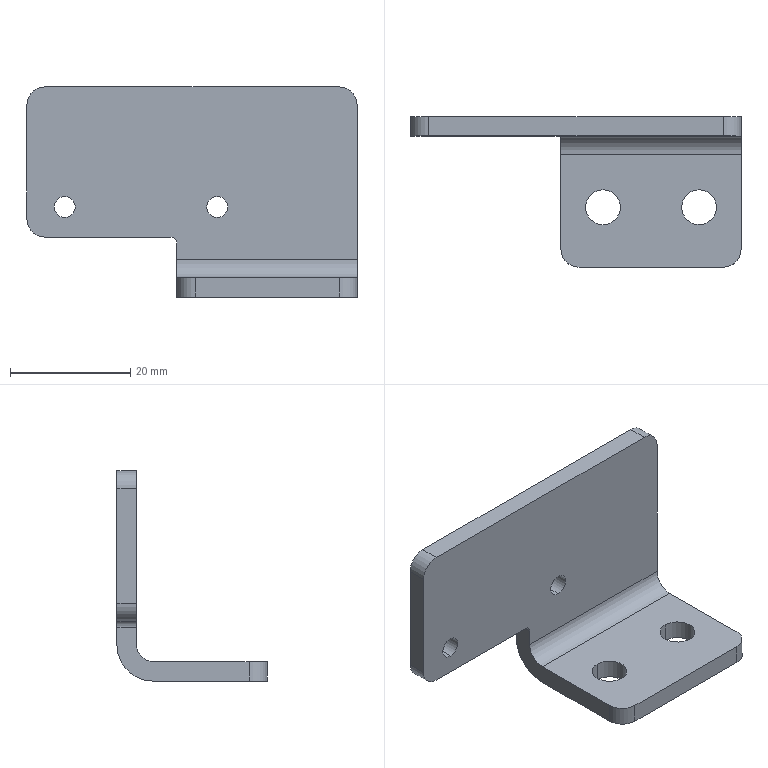Part | STEP file | J014-EBZ05-14-06-Part-1 | 1 solid | 26 faces | box 55 x 25 x 35 mm | volume 7018 mm3 | cylinder 16 | plane 10 | commonest cylinder face diameters 6 x6 3.5 x4 5.8 x4 2 x1 12 x1
STEP:
#1=CARTESIAN_POINT('',(-23.3,0.,13.25));
#2=VERTEX_POINT('',#1);
#3=CARTESIAN_POINT('',(-23.3,0.,16.75));
#4=VERTEX_POINT('',#3);
#5=CARTESIAN_POINT('',(-23.3,0.,15.));
#6=DIRECTION('',(0.,-1.,0.));
#7=DIRECTION('',(0.,0.,1.));
#8=AXIS2_PLACEMENT_3D('',#5,#6,#7);
#9=CIRCLE('',#8,1.75);
#10=EDGE_CURVE('',#2,#4,#9,.T.);
#11=ORIENTED_EDGE('',*,*,#10,.F.);
#12=CARTESIAN_POINT('',(-23.3,-3.2,13.25));
#13=VERTEX_POINT('',#12);
#14=CARTESIAN_POINT('',(-23.3,0.,13.25));
#15=DIRECTION('',(0.,-1.,0.));
#16=VECTOR('',#15,1000.);
#17=LINE('',#14,#16);
#18=EDGE_CURVE('',#2,#13,#17,.T.);
#19=ORIENTED_EDGE('',*,*,#18,.T.);
#20=CARTESIAN_POINT('',(-23.3,-3.2,16.75));
#21=VERTEX_POINT('',#20);
#22=CARTESIAN_POINT('',(-23.3,-3.2,15.));
#23=DIRECTION('',(0.,1.,0.));
#24=DIRECTION('',(0.,0.,-1.));
#25=AXIS2_PLACEMENT_3D('',#22,#23,#24);
#26=CIRCLE('',#25,1.75);
#27=EDGE_CURVE('',#21,#13,#26,.T.);
#28=ORIENTED_EDGE('',*,*,#27,.F.);
#29=CARTESIAN_POINT('',(-23.3,0.,16.75));
#30=DIRECTION('',(0.,-1.,0.));
#31=VECTOR('',#30,1000.);
#32=LINE('',#29,#31);
#33=EDGE_CURVE('',#4,#21,#32,.T.);
#34=ORIENTED_EDGE('',*,*,#33,.F.);
#35=EDGE_LOOP('',(#11,#19,#28,#34));
#36=FACE_OUTER_BOUND('',#35,.T.);
#37=CARTESIAN_POINT('',(-23.3,0.,15.));
#38=DIRECTION('',(0.,-1.,0.));
#39=DIRECTION('',(0.,0.,1.));
#40=AXIS2_PLACEMENT_3D('',#37,#38,#39);
#41=CYLINDRICAL_SURFACE('',#40,1.75);
#42=ADVANCED_FACE('',(#36),#41,.F.);
#43=CARTESIAN_POINT('',(-48.7,0.,13.25));
#44=VERTEX_POINT('',#43);
#45=CARTESIAN_POINT('',(-48.7,0.,16.75));
#46=VERTEX_POINT('',#45);
#47=CARTESIAN_POINT('',(-48.7,0.,15.));
#48=DIRECTION('',(0.,-1.,0.));
#49=DIRECTION('',(0.,0.,1.));
#50=AXIS2_PLACEMENT_3D('',#47,#48,#49);
#51=CIRCLE('',#50,1.75);
#52=EDGE_CURVE('',#44,#46,#51,.T.);
#53=ORIENTED_EDGE('',*,*,#52,.F.);
#54=CARTESIAN_POINT('',(-48.7,-3.2,13.25));
#55=VERTEX_POINT('',#54);
#56=CARTESIAN_POINT('',(-48.7,0.,13.25));
#57=DIRECTION('',(0.,-1.,0.));
#58=VECTOR('',#57,1000.);
#59=LINE('',#56,#58);
#60=EDGE_CURVE('',#44,#55,#59,.T.);
#61=ORIENTED_EDGE('',*,*,#60,.T.);
#62=CARTESIAN_POINT('',(-48.7,-3.2,16.75));
#63=VERTEX_POINT('',#62);
#64=CARTESIAN_POINT('',(-48.7,-3.2,15.));
#65=DIRECTION('',(0.,1.,0.));
#66=DIRECTION('',(0.,0.,-1.));
#67=AXIS2_PLACEMENT_3D('',#64,#65,#66);
#68=CIRCLE('',#67,1.75);
#69=EDGE_CURVE('',#63,#55,#68,.T.);
#70=ORIENTED_EDGE('',*,*,#69,.F.);
#71=CARTESIAN_POINT('',(-48.7,0.,16.75));
#72=DIRECTION('',(0.,-1.,0.));
#73=VECTOR('',#72,1000.);
#74=LINE('',#71,#73);
#75=EDGE_CURVE('',#46,#63,#74,.T.);
#76=ORIENTED_EDGE('',*,*,#75,.F.);
#77=EDGE_LOOP('',(#53,#61,#70,#76));
#78=FACE_OUTER_BOUND('',#77,.T.);
#79=CARTESIAN_POINT('',(-48.7,0.,15.));
#80=DIRECTION('',(0.,-1.,0.));
#81=DIRECTION('',(0.,0.,1.));
#82=AXIS2_PLACEMENT_3D('',#79,#80,#81);
#83=CYLINDRICAL_SURFACE('',#82,1.75);
#84=ADVANCED_FACE('',(#78),#83,.F.);
#85=CARTESIAN_POINT('',(-7.,-12.1,3.2));
#86=VERTEX_POINT('',#85);
#87=CARTESIAN_POINT('',(-7.,-17.9,3.2));
#88=VERTEX_POINT('',#87);
#89=CARTESIAN_POINT('',(-7.,-15.,3.2));
#90=DIRECTION('',(0.,0.,-1.));
#91=DIRECTION('',(0.,-1.,0.));
#92=AXIS2_PLACEMENT_3D('',#89,#90,#91);
#93=CIRCLE('',#92,2.9);
#94=EDGE_CURVE('',#86,#88,#93,.T.);
#95=ORIENTED_EDGE('',*,*,#94,.F.);
#96=CARTESIAN_POINT('',(-7.,-12.1,0.));
#97=VERTEX_POINT('',#96);
#98=CARTESIAN_POINT('',(-7.,-12.1,3.2));
#99=DIRECTION('',(0.,0.,-1.));
#100=VECTOR('',#99,1000.);
#101=LINE('',#98,#100);
#102=EDGE_CURVE('',#86,#97,#101,.T.);
#103=ORIENTED_EDGE('',*,*,#102,.T.);
#104=CARTESIAN_POINT('',(-7.,-17.9,0.));
#105=VERTEX_POINT('',#104);
#106=CARTESIAN_POINT('',(-7.,-15.,0.));
#107=DIRECTION('',(0.,0.,-1.));
#108=DIRECTION('',(0.,-1.,0.));
#109=AXIS2_PLACEMENT_3D('',#106,#107,#108);
#110=CIRCLE('',#109,2.9);
#111=EDGE_CURVE('',#97,#105,#110,.T.);
#112=ORIENTED_EDGE('',*,*,#111,.T.);
#113=CARTESIAN_POINT('',(-7.,-17.9,3.2));
#114=DIRECTION('',(0.,0.,-1.));
#115=VECTOR('',#114,1000.);
#116=LINE('',#113,#115);
#117=EDGE_CURVE('',#88,#105,#116,.T.);
#118=ORIENTED_EDGE('',*,*,#117,.F.);
#119=EDGE_LOOP('',(#95,#103,#112,#118));
#120=FACE_OUTER_BOUND('',#119,.T.);
#121=CARTESIAN_POINT('',(-7.,-15.,3.2));
#122=DIRECTION('',(0.,0.,-1.));
#123=DIRECTION('',(0.,-1.,0.));
#124=AXIS2_PLACEMENT_3D('',#121,#122,#123);
#125=CYLINDRICAL_SURFACE('',#124,2.9);
#126=ADVANCED_FACE('',(#120),#125,.F.);
#127=CARTESIAN_POINT('',(-23.,-12.1,3.2));
#128=VERTEX_POINT('',#127);
#129=CARTESIAN_POINT('',(-23.,-17.9,3.2));
#130=VERTEX_POINT('',#129);
#131=CARTESIAN_POINT('',(-23.,-15.,3.2));
#132=DIRECTION('',(0.,0.,-1.));
#133=DIRECTION('',(0.,-1.,0.));
#134=AXIS2_PLACEMENT_3D('',#131,#132,#133);
#135=CIRCLE('',#134,2.9);
#136=EDGE_CURVE('',#128,#130,#135,.T.);
#137=ORIENTED_EDGE('',*,*,#136,.F.);
#138=CARTESIAN_POINT('',(-23.,-12.1,0.));
#139=VERTEX_POINT('',#138);
#140=CARTESIAN_POINT('',(-23.,-12.1,3.2));
#141=DIRECTION('',(0.,0.,-1.));
#142=VECTOR('',#141,1000.);
#143=LINE('',#140,#142);
#144=EDGE_CURVE('',#128,#139,#143,.T.);
#145=ORIENTED_EDGE('',*,*,#144,.T.);
#146=CARTESIAN_POINT('',(-23.,-17.9,0.));
#147=VERTEX_POINT('',#146);
#148=CARTESIAN_POINT('',(-23.,-15.,0.));
#149=DIRECTION('',(0.,0.,-1.));
#150=DIRECTION('',(0.,-1.,0.));
#151=AXIS2_PLACEMENT_3D('',#148,#149,#150);
#152=CIRCLE('',#151,2.9);
#153=EDGE_CURVE('',#139,#147,#152,.T.);
#154=ORIENTED_EDGE('',*,*,#153,.T.);
#155=CARTESIAN_POINT('',(-23.,-17.9,3.2));
#156=DIRECTION('',(0.,0.,-1.));
#157=VECTOR('',#156,1000.);
#158=LINE('',#155,#157);
#159=EDGE_CURVE('',#130,#147,#158,.T.);
#160=ORIENTED_EDGE('',*,*,#159,.F.);
#161=EDGE_LOOP('',(#137,#145,#154,#160));
#162=FACE_OUTER_BOUND('',#161,.T.);
#163=CARTESIAN_POINT('',(-23.,-15.,3.2));
#164=DIRECTION('',(0.,0.,-1.));
#165=DIRECTION('',(0.,-1.,0.));
#166=AXIS2_PLACEMENT_3D('',#163,#164,#165);
#167=CYLINDRICAL_SURFACE('',#166,2.9);
#168=ADVANCED_FACE('',(#162),#167,.F.);
#169=CARTESIAN_POINT('',(-30.,-3.2,6.2));
#170=VERTEX_POINT('',#169);
#171=CARTESIAN_POINT('',(-30.,-3.2,9.));
#172=VERTEX_POINT('',#171);
#173=CARTESIAN_POINT('',(-30.,-3.2,3.2));
#174=DIRECTION('',(0.,0.,1.));
#175=VECTOR('',#174,1000.);
#176=LINE('',#173,#175);
#177=EDGE_CURVE('',#170,#172,#176,.T.);
#178=ORIENTED_EDGE('',*,*,#177,.T.);
#179=CARTESIAN_POINT('',(-30.,0.,9.));
#180=VERTEX_POINT('',#179);
#181=CARTESIAN_POINT('',(-30.,0.,9.));
#182=DIRECTION('',(0.,1.,0.));
#183=VECTOR('',#182,1000.);
#184=LINE('',#181,#183);
#185=EDGE_CURVE('',#172,#180,#184,.T.);
#186=ORIENTED_EDGE('',*,*,#185,.T.);
#187=CARTESIAN_POINT('',(-30.,0.,6.));
#188=VERTEX_POINT('',#187);
#189=CARTESIAN_POINT('',(-30.,0.,0.));
#190=DIRECTION('',(0.,0.,1.));
#191=VECTOR('',#190,1000.);
#192=LINE('',#189,#191);
#193=EDGE_CURVE('',#188,#180,#192,.T.);
#194=ORIENTED_EDGE('',*,*,#193,.F.);
#195=CARTESIAN_POINT('',(-30.,-6.,0.));
#196=VERTEX_POINT('',#195);
#197=CARTESIAN_POINT('',(-30.,-6.,6.));
#198=DIRECTION('',(-1.,0.,0.));
#199=DIRECTION('',(0.,0.,-1.));
#200=AXIS2_PLACEMENT_3D('',#197,#198,#199);
#201=CIRCLE('',#200,6.);
#202=EDGE_CURVE('',#188,#196,#201,.T.);
#203=ORIENTED_EDGE('',*,*,#202,.T.);
#204=CARTESIAN_POINT('',(-30.,-22.,0.));
#205=VERTEX_POINT('',#204);
#206=CARTESIAN_POINT('',(-30.,-12.5,0.));
#207=DIRECTION('',(0.,-1.,0.));
#208=VECTOR('',#207,1000.);
#209=LINE('',#206,#208);
#210=EDGE_CURVE('',#196,#205,#209,.T.);
#211=ORIENTED_EDGE('',*,*,#210,.T.);
#212=CARTESIAN_POINT('',(-30.,-22.,3.2));
#213=VERTEX_POINT('',#212);
#214=CARTESIAN_POINT('',(-30.,-22.,0.));
#215=DIRECTION('',(0.,0.,1.));
#216=VECTOR('',#215,1000.);
#217=LINE('',#214,#216);
#218=EDGE_CURVE('',#205,#213,#217,.T.);
#219=ORIENTED_EDGE('',*,*,#218,.T.);
#220=CARTESIAN_POINT('',(-30.,-6.2,3.2));
#221=VERTEX_POINT('',#220);
#222=CARTESIAN_POINT('',(-30.,-12.5,3.2));
#223=DIRECTION('',(0.,1.,0.));
#224=VECTOR('',#223,1000.);
#225=LINE('',#222,#224);
#226=EDGE_CURVE('',#213,#221,#225,.T.);
#227=ORIENTED_EDGE('',*,*,#226,.T.);
#228=CARTESIAN_POINT('',(-30.,-6.2,6.2));
#229=DIRECTION('',(1.,0.,0.));
#230=DIRECTION('',(0.,0.,-1.));
#231=AXIS2_PLACEMENT_3D('',#228,#229,#230);
#232=CIRCLE('',#231,3.);
#233=EDGE_CURVE('',#221,#170,#232,.T.);
#234=ORIENTED_EDGE('',*,*,#233,.T.);
#235=EDGE_LOOP('',(#178,#186,#194,#203,#211,#219,#227,#234));
#236=FACE_OUTER_BOUND('',#235,.T.);
#237=CARTESIAN_POINT('',(-30.,-12.5,0.));
#238=DIRECTION('',(-1.,0.,0.));
#239=DIRECTION('',(0.,0.,1.));
#240=AXIS2_PLACEMENT_3D('',#237,#238,#239);
#241=PLANE('',#240);
#242=ADVANCED_FACE('',(#236),#241,.T.);
#243=CARTESIAN_POINT('',(-7.,-15.,3.2));
#244=DIRECTION('',(0.,0.,-1.));
#245=DIRECTION('',(0.,-1.,0.));
#246=AXIS2_PLACEMENT_3D('',#243,#244,#245);
#247=CIRCLE('',#246,2.9);
#248=EDGE_CURVE('',#88,#86,#247,.T.);
#249=ORIENTED_EDGE('',*,*,#248,.T.);
#250=ORIENTED_EDGE('',*,*,#94,.T.);
#251=EDGE_LOOP('',(#249,#250));
#252=FACE_BOUND('',#251,.T.);
#253=CARTESIAN_POINT('',(-23.,-15.,3.2));
#254=DIRECTION('',(0.,0.,-1.));
#255=DIRECTION('',(0.,-1.,0.));
#256=AXIS2_PLACEMENT_3D('',#253,#254,#255);
#257=CIRCLE('',#256,2.9);
#258=EDGE_CURVE('',#130,#128,#257,.T.);
#259=ORIENTED_EDGE('',*,*,#258,.T.);
#260=ORIENTED_EDGE('',*,*,#136,.T.);
#261=EDGE_LOOP('',(#259,#260));
#262=FACE_BOUND('',#261,.T.);
#263=ORIENTED_EDGE('',*,*,#226,.F.);
#264=CARTESIAN_POINT('',(-27.,-25.,3.2));
#265=VERTEX_POINT('',#264);
#266=CARTESIAN_POINT('',(-27.,-22.,3.2));
#267=DIRECTION('',(0.,0.,1.));
#268=DIRECTION('',(0.,1.,0.));
#269=AXIS2_PLACEMENT_3D('',#266,#267,#268);
#270=CIRCLE('',#269,3.);
#271=EDGE_CURVE('',#213,#265,#270,.T.);
#272=ORIENTED_EDGE('',*,*,#271,.T.);
#273=CARTESIAN_POINT('',(-3.,-25.,3.2));
#274=VERTEX_POINT('',#273);
#275=CARTESIAN_POINT('',(-15.,-25.,3.2));
#276=DIRECTION('',(-1.,0.,0.));
#277=VECTOR('',#276,1000.);
#278=LINE('',#275,#277);
#279=EDGE_CURVE('',#274,#265,#278,.T.);
#280=ORIENTED_EDGE('',*,*,#279,.F.);
#281=CARTESIAN_POINT('',(0.,-22.,3.2));
#282=VERTEX_POINT('',#281);
#283=CARTESIAN_POINT('',(-3.,-22.,3.2));
#284=DIRECTION('',(0.,0.,1.));
#285=DIRECTION('',(0.,1.,0.));
#286=AXIS2_PLACEMENT_3D('',#283,#284,#285);
#287=CIRCLE('',#286,3.);
#288=EDGE_CURVE('',#274,#282,#287,.T.);
#289=ORIENTED_EDGE('',*,*,#288,.T.);
#290=CARTESIAN_POINT('',(0.,-6.2,3.2));
#291=VERTEX_POINT('',#290);
#292=CARTESIAN_POINT('',(0.,-12.5,3.2));
#293=DIRECTION('',(0.,-1.,0.));
#294=VECTOR('',#293,1000.);
#295=LINE('',#292,#294);
#296=EDGE_CURVE('',#291,#282,#295,.T.);
#297=ORIENTED_EDGE('',*,*,#296,.F.);
#298=CARTESIAN_POINT('',(-30.,-6.2,3.2));
#299=DIRECTION('',(-1.,0.,0.));
#300=VECTOR('',#299,1000.);
#301=LINE('',#298,#300);
#302=EDGE_CURVE('',#291,#221,#301,.T.);
#303=ORIENTED_EDGE('',*,*,#302,.T.);
#304=EDGE_LOOP('',(#263,#272,#280,#289,#297,#303));
#305=FACE_OUTER_BOUND('',#304,.T.);
#306=CARTESIAN_POINT('',(-15.,-12.5,3.2));
#307=DIRECTION('',(0.,0.,1.));
#308=DIRECTION('',(0.,1.,0.));
#309=AXIS2_PLACEMENT_3D('',#306,#307,#308);
#310=PLANE('',#309);
#311=ADVANCED_FACE('',(#252,#262,#305),#310,.T.);
#312=CARTESIAN_POINT('',(0.,0.,6.));
#313=VERTEX_POINT('',#312);
#314=CARTESIAN_POINT('',(0.,0.,32.));
#315=VERTEX_POINT('',#314);
#316=CARTESIAN_POINT('',(0.,0.,0.));
#317=DIRECTION('',(0.,0.,1.));
#318=VECTOR('',#317,1000.);
#319=LINE('',#316,#318);
#320=EDGE_CURVE('',#313,#315,#319,.T.);
#321=ORIENTED_EDGE('',*,*,#320,.T.);
#322=CARTESIAN_POINT('',(0.,-3.2,32.));
#323=VERTEX_POINT('',#322);
#324=CARTESIAN_POINT('',(0.,-12.5,32.));
#325=DIRECTION('',(0.,-1.,0.));
#326=VECTOR('',#325,1000.);
#327=LINE('',#324,#326);
#328=EDGE_CURVE('',#315,#323,#327,.T.);
#329=ORIENTED_EDGE('',*,*,#328,.T.);
#330=CARTESIAN_POINT('',(0.,-3.2,6.2));
#331=VERTEX_POINT('',#330);
#332=CARTESIAN_POINT('',(0.,-3.2,3.2));
#333=DIRECTION('',(0.,0.,1.));
#334=VECTOR('',#333,1000.);
#335=LINE('',#332,#334);
#336=EDGE_CURVE('',#331,#323,#335,.T.);
#337=ORIENTED_EDGE('',*,*,#336,.F.);
#338=CARTESIAN_POINT('',(0.,-6.2,6.2));
#339=DIRECTION('',(-1.,0.,0.));
#340=DIRECTION('',(0.,0.,1.));
#341=AXIS2_PLACEMENT_3D('',#338,#339,#340);
#342=CIRCLE('',#341,3.);
#343=EDGE_CURVE('',#331,#291,#342,.T.);
#344=ORIENTED_EDGE('',*,*,#343,.T.);
#345=ORIENTED_EDGE('',*,*,#296,.T.);
#346=CARTESIAN_POINT('',(0.,-22.,0.));
#347=VERTEX_POINT('',#346);
#348=CARTESIAN_POINT('',(0.,-22.,0.));
#349=DIRECTION('',(0.,0.,-1.));
#350=VECTOR('',#349,1000.);
#351=LINE('',#348,#350);
#352=EDGE_CURVE('',#282,#347,#351,.T.);
#353=ORIENTED_EDGE('',*,*,#352,.T.);
#354=CARTESIAN_POINT('',(0.,-6.,0.));
#355=VERTEX_POINT('',#354);
#356=CARTESIAN_POINT('',(0.,-12.5,0.));
#357=DIRECTION('',(0.,1.,0.));
#358=VECTOR('',#357,1000.);
#359=LINE('',#356,#358);
#360=EDGE_CURVE('',#347,#355,#359,.T.);
#361=ORIENTED_EDGE('',*,*,#360,.T.);
#362=CARTESIAN_POINT('',(0.,-6.,6.));
#363=DIRECTION('',(1.,0.,0.));
#364=DIRECTION('',(0.,0.,1.));
#365=AXIS2_PLACEMENT_3D('',#362,#363,#364);
#366=CIRCLE('',#365,6.);
#367=EDGE_CURVE('',#355,#313,#366,.T.);
#368=ORIENTED_EDGE('',*,*,#367,.T.);
#369=EDGE_LOOP('',(#321,#329,#337,#344,#345,#353,#361,#368));
#370=FACE_OUTER_BOUND('',#369,.T.);
#371=CARTESIAN_POINT('',(0.,-12.5,0.));
#372=DIRECTION('',(1.,0.,0.));
#373=DIRECTION('',(0.,0.,-1.));
#374=AXIS2_PLACEMENT_3D('',#371,#372,#373);
#375=PLANE('',#374);
#376=ADVANCED_FACE('',(#370),#375,.T.);
#377=ORIENTED_EDGE('',*,*,#279,.T.);
#378=CARTESIAN_POINT('',(-27.,-25.,0.));
#379=VERTEX_POINT('',#378);
#380=CARTESIAN_POINT('',(-27.,-25.,0.));
#381=DIRECTION('',(0.,0.,-1.));
#382=VECTOR('',#381,1000.);
#383=LINE('',#380,#382);
#384=EDGE_CURVE('',#265,#379,#383,.T.);
#385=ORIENTED_EDGE('',*,*,#384,.T.);
#386=CARTESIAN_POINT('',(-3.,-25.,0.));
#387=VERTEX_POINT('',#386);
#388=CARTESIAN_POINT('',(-15.,-25.,0.));
#389=DIRECTION('',(1.,0.,0.));
#390=VECTOR('',#389,1000.);
#391=LINE('',#388,#390);
#392=EDGE_CURVE('',#379,#387,#391,.T.);
#393=ORIENTED_EDGE('',*,*,#392,.T.);
#394=CARTESIAN_POINT('',(-3.,-25.,0.));
#395=DIRECTION('',(0.,0.,1.));
#396=VECTOR('',#395,1000.);
#397=LINE('',#394,#396);
#398=EDGE_CURVE('',#387,#274,#397,.T.);
#399=ORIENTED_EDGE('',*,*,#398,.T.);
#400=EDGE_LOOP('',(#377,#385,#393,#399));
#401=FACE_OUTER_BOUND('',#400,.T.);
#402=CARTESIAN_POINT('',(-15.,-25.,0.));
#403=DIRECTION('',(0.,-1.,0.));
#404=DIRECTION('',(0.,0.,1.));
#405=AXIS2_PLACEMENT_3D('',#402,#403,#404);
#406=PLANE('',#405);
#407=ADVANCED_FACE('',(#401),#406,.T.);
#408=CARTESIAN_POINT('',(-7.,-15.,0.));
#409=DIRECTION('',(0.,0.,-1.));
#410=DIRECTION('',(0.,-1.,0.));
#411=AXIS2_PLACEMENT_3D('',#408,#409,#410);
#412=CIRCLE('',#411,2.9);
#413=EDGE_CURVE('',#105,#97,#412,.T.);
#414=ORIENTED_EDGE('',*,*,#413,.F.);
#415=ORIENTED_EDGE('',*,*,#111,.F.);
#416=EDGE_LOOP('',(#414,#415));
#417=FACE_BOUND('',#416,.T.);
#418=CARTESIAN_POINT('',(-23.,-15.,0.));
#419=DIRECTION('',(0.,0.,-1.));
#420=DIRECTION('',(0.,-1.,0.));
#421=AXIS2_PLACEMENT_3D('',#418,#419,#420);
#422=CIRCLE('',#421,2.9);
#423=EDGE_CURVE('',#147,#139,#422,.T.);
#424=ORIENTED_EDGE('',*,*,#423,.F.);
#425=ORIENTED_EDGE('',*,*,#153,.F.);
#426=EDGE_LOOP('',(#424,#425));
#427=FACE_BOUND('',#426,.T.);
#428=ORIENTED_EDGE('',*,*,#392,.F.);
#429=CARTESIAN_POINT('',(-27.,-22.,0.));
#430=DIRECTION('',(0.,0.,-1.));
#431=DIRECTION('',(0.,-1.,0.));
#432=AXIS2_PLACEMENT_3D('',#429,#430,#431);
#433=CIRCLE('',#432,3.);
#434=EDGE_CURVE('',#379,#205,#433,.T.);
#435=ORIENTED_EDGE('',*,*,#434,.T.);
#436=ORIENTED_EDGE('',*,*,#210,.F.);
#437=CARTESIAN_POINT('',(-15.,-6.,0.));
#438=DIRECTION('',(1.,0.,0.));
#439=VECTOR('',#438,1000.);
#440=LINE('',#437,#439);
#441=EDGE_CURVE('',#196,#355,#440,.T.);
#442=ORIENTED_EDGE('',*,*,#441,.T.);
#443=ORIENTED_EDGE('',*,*,#360,.F.);
#444=CARTESIAN_POINT('',(-3.,-22.,0.));
#445=DIRECTION('',(0.,0.,-1.));
#446=DIRECTION('',(0.,-1.,0.));
#447=AXIS2_PLACEMENT_3D('',#444,#445,#446);
#448=CIRCLE('',#447,3.);
#449=EDGE_CURVE('',#347,#387,#448,.T.);
#450=ORIENTED_EDGE('',*,*,#449,.T.);
#451=EDGE_LOOP('',(#428,#435,#436,#442,#443,#450));
#452=FACE_OUTER_BOUND('',#451,.T.);
#453=CARTESIAN_POINT('',(-15.,-12.5,0.));
#454=DIRECTION('',(0.,0.,-1.));
#455=DIRECTION('',(0.,-1.,0.));
#456=AXIS2_PLACEMENT_3D('',#453,#454,#455);
#457=PLANE('',#456);
#458=ADVANCED_FACE('',(#417,#427,#452),#457,.T.);
#459=CARTESIAN_POINT('',(-23.3,0.,15.));
#460=DIRECTION('',(0.,-1.,0.));
#461=DIRECTION('',(0.,0.,1.));
#462=AXIS2_PLACEMENT_3D('',#459,#460,#461);
#463=CIRCLE('',#462,1.75);
#464=EDGE_CURVE('',#4,#2,#463,.T.);
#465=ORIENTED_EDGE('',*,*,#464,.T.);
#466=ORIENTED_EDGE('',*,*,#10,.T.);
#467=EDGE_LOOP('',(#465,#466));
#468=FACE_BOUND('',#467,.T.);
#469=CARTESIAN_POINT('',(-48.7,0.,15.));
#470=DIRECTION('',(0.,-1.,0.));
#471=DIRECTION('',(0.,0.,1.));
#472=AXIS2_PLACEMENT_3D('',#469,#470,#471);
#473=CIRCLE('',#472,1.75);
#474=EDGE_CURVE('',#46,#44,#473,.T.);
#475=ORIENTED_EDGE('',*,*,#474,.T.);
#476=ORIENTED_EDGE('',*,*,#52,.T.);
#477=EDGE_LOOP('',(#475,#476));
#478=FACE_BOUND('',#477,.T.);
#479=CARTESIAN_POINT('',(-52.,0.,10.));
#480=VERTEX_POINT('',#479);
#481=CARTESIAN_POINT('',(-31.,0.,10.));
#482=VERTEX_POINT('',#481);
#483=CARTESIAN_POINT('',(-42.5,0.,10.));
#484=DIRECTION('',(1.,0.,0.));
#485=VECTOR('',#484,1000.);
#486=LINE('',#483,#485);
#487=EDGE_CURVE('',#480,#482,#486,.T.);
#488=ORIENTED_EDGE('',*,*,#487,.F.);
#489=CARTESIAN_POINT('',(-55.,0.,13.));
#490=VERTEX_POINT('',#489);
#491=CARTESIAN_POINT('',(-52.,0.,13.));
#492=DIRECTION('',(0.,1.,0.));
#493=DIRECTION('',(0.,0.,-1.));
#494=AXIS2_PLACEMENT_3D('',#491,#492,#493);
#495=CIRCLE('',#494,3.);
#496=EDGE_CURVE('',#480,#490,#495,.T.);
#497=ORIENTED_EDGE('',*,*,#496,.T.);
#498=CARTESIAN_POINT('',(-55.,0.,32.));
#499=VERTEX_POINT('',#498);
#500=CARTESIAN_POINT('',(-55.,0.,22.5));
#501=DIRECTION('',(0.,0.,-1.));
#502=VECTOR('',#501,1000.);
#503=LINE('',#500,#502);
#504=EDGE_CURVE('',#499,#490,#503,.T.);
#505=ORIENTED_EDGE('',*,*,#504,.F.);
#506=CARTESIAN_POINT('',(-52.,0.,35.));
#507=VERTEX_POINT('',#506);
#508=CARTESIAN_POINT('',(-52.,0.,32.));
#509=DIRECTION('',(0.,1.,0.));
#510=DIRECTION('',(0.,0.,-1.));
#511=AXIS2_PLACEMENT_3D('',#508,#509,#510);
#512=CIRCLE('',#511,3.);
#513=EDGE_CURVE('',#499,#507,#512,.T.);
#514=ORIENTED_EDGE('',*,*,#513,.T.);
#515=CARTESIAN_POINT('',(-3.,0.,35.));
#516=VERTEX_POINT('',#515);
#517=CARTESIAN_POINT('',(-15.,0.,35.));
#518=DIRECTION('',(1.,0.,0.));
#519=VECTOR('',#518,1000.);
#520=LINE('',#517,#519);
#521=EDGE_CURVE('',#507,#516,#520,.T.);
#522=ORIENTED_EDGE('',*,*,#521,.T.);
#523=CARTESIAN_POINT('',(-3.,0.,32.));
#524=DIRECTION('',(0.,1.,0.));
#525=DIRECTION('',(0.,0.,-1.));
#526=AXIS2_PLACEMENT_3D('',#523,#524,#525);
#527=CIRCLE('',#526,3.);
#528=EDGE_CURVE('',#516,#315,#527,.T.);
#529=ORIENTED_EDGE('',*,*,#528,.T.);
#530=ORIENTED_EDGE('',*,*,#320,.F.);
#531=CARTESIAN_POINT('',(-15.,0.,6.));
#532=DIRECTION('',(-1.,0.,0.));
#533=VECTOR('',#532,1000.);
#534=LINE('',#531,#533);
#535=EDGE_CURVE('',#313,#188,#534,.T.);
#536=ORIENTED_EDGE('',*,*,#535,.T.);
#537=ORIENTED_EDGE('',*,*,#193,.T.);
#538=CARTESIAN_POINT('',(-31.,0.,9.));
#539=DIRECTION('',(0.,-1.,0.));
#540=DIRECTION('',(0.,0.,-1.));
#541=AXIS2_PLACEMENT_3D('',#538,#539,#540);
#542=CIRCLE('',#541,1.);
#543=EDGE_CURVE('',#180,#482,#542,.T.);
#544=ORIENTED_EDGE('',*,*,#543,.T.);
#545=EDGE_LOOP('',(#488,#497,#505,#514,#522,#529,#530,#536,#537,#544));
#546=FACE_OUTER_BOUND('',#545,.T.);
#547=CARTESIAN_POINT('',(-15.,0.,0.));
#548=DIRECTION('',(0.,1.,0.));
#549=DIRECTION('',(0.,0.,-1.));
#550=AXIS2_PLACEMENT_3D('',#547,#548,#549);
#551=PLANE('',#550);
#552=ADVANCED_FACE('',(#468,#478,#546),#551,.T.);
#553=ORIENTED_EDGE('',*,*,#521,.F.);
#554=CARTESIAN_POINT('',(-52.,-3.2,35.));
#555=VERTEX_POINT('',#554);
#556=CARTESIAN_POINT('',(-52.,-1.6,35.));
#557=DIRECTION('',(0.,-1.,0.));
#558=VECTOR('',#557,1000.);
#559=LINE('',#556,#558);
#560=EDGE_CURVE('',#507,#555,#559,.T.);
#561=ORIENTED_EDGE('',*,*,#560,.T.);
#562=CARTESIAN_POINT('',(-3.,-3.2,35.));
#563=VERTEX_POINT('',#562);
#564=CARTESIAN_POINT('',(-15.,-3.2,35.));
#565=DIRECTION('',(-1.,0.,0.));
#566=VECTOR('',#565,1000.);
#567=LINE('',#564,#566);
#568=EDGE_CURVE('',#563,#555,#567,.T.);
#569=ORIENTED_EDGE('',*,*,#568,.F.);
#570=CARTESIAN_POINT('',(-3.,-1.6,35.));
#571=DIRECTION('',(0.,1.,0.));
#572=VECTOR('',#571,1000.);
#573=LINE('',#570,#572);
#574=EDGE_CURVE('',#563,#516,#573,.T.);
#575=ORIENTED_EDGE('',*,*,#574,.T.);
#576=EDGE_LOOP('',(#553,#561,#569,#575));
#577=FACE_OUTER_BOUND('',#576,.T.);
#578=CARTESIAN_POINT('',(-15.,-1.6,35.));
#579=DIRECTION('',(0.,0.,1.));
#580=DIRECTION('',(0.,-1.,0.));
#581=AXIS2_PLACEMENT_3D('',#578,#579,#580);
#582=PLANE('',#581);
#583=ADVANCED_FACE('',(#577),#582,.T.);
#584=ORIENTED_EDGE('',*,*,#27,.T.);
#585=CARTESIAN_POINT('',(-23.3,-3.2,15.));
#586=DIRECTION('',(0.,1.,0.));
#587=DIRECTION('',(0.,0.,-1.));
#588=AXIS2_PLACEMENT_3D('',#585,#586,#587);
#589=CIRCLE('',#588,1.75);
#590=EDGE_CURVE('',#13,#21,#589,.T.);
#591=ORIENTED_EDGE('',*,*,#590,.T.);
#592=EDGE_LOOP('',(#584,#591));
#593=FACE_BOUND('',#592,.T.);
#594=ORIENTED_EDGE('',*,*,#69,.T.);
#595=CARTESIAN_POINT('',(-48.7,-3.2,15.));
#596=DIRECTION('',(0.,1.,0.));
#597=DIRECTION('',(0.,0.,-1.));
#598=AXIS2_PLACEMENT_3D('',#595,#596,#597);
#599=CIRCLE('',#598,1.75);
#600=EDGE_CURVE('',#55,#63,#599,.T.);
#601=ORIENTED_EDGE('',*,*,#600,.T.);
#602=EDGE_LOOP('',(#594,#601));
#603=FACE_BOUND('',#602,.T.);
#604=CARTESIAN_POINT('',(-55.,-3.2,13.));
#605=VERTEX_POINT('',#604);
#606=CARTESIAN_POINT('',(-55.,-3.2,32.));
#607=VERTEX_POINT('',#606);
#608=CARTESIAN_POINT('',(-55.,-3.2,22.5));
#609=DIRECTION('',(0.,0.,1.));
#610=VECTOR('',#609,1000.);
#611=LINE('',#608,#610);
#612=EDGE_CURVE('',#605,#607,#611,.T.);
#613=ORIENTED_EDGE('',*,*,#612,.F.);
#614=CARTESIAN_POINT('',(-52.,-3.2,10.));
#615=VERTEX_POINT('',#614);
#616=CARTESIAN_POINT('',(-52.,-3.2,13.));
#617=DIRECTION('',(0.,-1.,0.));
#618=DIRECTION('',(0.,0.,1.));
#619=AXIS2_PLACEMENT_3D('',#616,#617,#618);
#620=CIRCLE('',#619,3.);
#621=EDGE_CURVE('',#605,#615,#620,.T.);
#622=ORIENTED_EDGE('',*,*,#621,.T.);
#623=CARTESIAN_POINT('',(-31.,-3.2,10.));
#624=VERTEX_POINT('',#623);
#625=CARTESIAN_POINT('',(-42.5,-3.2,10.));
#626=DIRECTION('',(-1.,0.,0.));
#627=VECTOR('',#626,1000.);
#628=LINE('',#625,#627);
#629=EDGE_CURVE('',#624,#615,#628,.T.);
#630=ORIENTED_EDGE('',*,*,#629,.F.);
#631=CARTESIAN_POINT('',(-31.,-3.2,9.));
#632=DIRECTION('',(0.,1.,0.));
#633=DIRECTION('',(0.,0.,1.));
#634=AXIS2_PLACEMENT_3D('',#631,#632,#633);
#635=CIRCLE('',#634,1.);
#636=EDGE_CURVE('',#624,#172,#635,.T.);
#637=ORIENTED_EDGE('',*,*,#636,.T.);
#638=ORIENTED_EDGE('',*,*,#177,.F.);
#639=CARTESIAN_POINT('',(0.,-3.2,6.2));
#640=DIRECTION('',(1.,0.,0.));
#641=VECTOR('',#640,1000.);
#642=LINE('',#639,#641);
#643=EDGE_CURVE('',#170,#331,#642,.T.);
#644=ORIENTED_EDGE('',*,*,#643,.T.);
#645=ORIENTED_EDGE('',*,*,#336,.T.);
#646=CARTESIAN_POINT('',(-3.,-3.2,32.));
#647=DIRECTION('',(0.,-1.,0.));
#648=DIRECTION('',(0.,0.,1.));
#649=AXIS2_PLACEMENT_3D('',#646,#647,#648);
#650=CIRCLE('',#649,3.);
#651=EDGE_CURVE('',#323,#563,#650,.T.);
#652=ORIENTED_EDGE('',*,*,#651,.T.);
#653=ORIENTED_EDGE('',*,*,#568,.T.);
#654=CARTESIAN_POINT('',(-52.,-3.2,32.));
#655=DIRECTION('',(0.,-1.,0.));
#656=DIRECTION('',(0.,0.,1.));
#657=AXIS2_PLACEMENT_3D('',#654,#655,#656);
#658=CIRCLE('',#657,3.);
#659=EDGE_CURVE('',#555,#607,#658,.T.);
#660=ORIENTED_EDGE('',*,*,#659,.T.);
#661=EDGE_LOOP('',(#613,#622,#630,#637,#638,#644,#645,#652,#653,#660));
#662=FACE_OUTER_BOUND('',#661,.T.);
#663=CARTESIAN_POINT('',(-15.,-3.2,3.2));
#664=DIRECTION('',(0.,-1.,0.));
#665=DIRECTION('',(0.,0.,-1.));
#666=AXIS2_PLACEMENT_3D('',#663,#664,#665);
#667=PLANE('',#666);
#668=ADVANCED_FACE('',(#593,#603,#662),#667,.T.);
#669=ORIENTED_EDGE('',*,*,#233,.F.);
#670=ORIENTED_EDGE('',*,*,#302,.F.);
#671=ORIENTED_EDGE('',*,*,#343,.F.);
#672=ORIENTED_EDGE('',*,*,#643,.F.);
#673=EDGE_LOOP('',(#669,#670,#671,#672));
#674=FACE_OUTER_BOUND('',#673,.T.);
#675=CARTESIAN_POINT('',(-15.,-6.2,6.2));
#676=DIRECTION('',(-1.,0.,0.));
#677=DIRECTION('',(0.,1.,0.));
#678=AXIS2_PLACEMENT_3D('',#675,#676,#677);
#679=CYLINDRICAL_SURFACE('',#678,3.);
#680=ADVANCED_FACE('',(#674),#679,.F.);
#681=ORIENTED_EDGE('',*,*,#367,.F.);
#682=ORIENTED_EDGE('',*,*,#441,.F.);
#683=ORIENTED_EDGE('',*,*,#202,.F.);
#684=ORIENTED_EDGE('',*,*,#535,.F.);
#685=EDGE_LOOP('',(#681,#682,#683,#684));
#686=FACE_OUTER_BOUND('',#685,.T.);
#687=CARTESIAN_POINT('',(-15.,-6.,6.));
#688=DIRECTION('',(-1.,0.,0.));
#689=DIRECTION('',(0.,0.,-1.));
#690=AXIS2_PLACEMENT_3D('',#687,#688,#689);
#691=CYLINDRICAL_SURFACE('',#690,6.);
#692=ADVANCED_FACE('',(#686),#691,.T.);
#693=ORIENTED_EDGE('',*,*,#449,.F.);
#694=ORIENTED_EDGE('',*,*,#352,.F.);
#695=ORIENTED_EDGE('',*,*,#288,.F.);
#696=ORIENTED_EDGE('',*,*,#398,.F.);
#697=EDGE_LOOP('',(#693,#694,#695,#696));
#698=FACE_OUTER_BOUND('',#697,.T.);
#699=CARTESIAN_POINT('',(-3.,-22.,0.));
#700=DIRECTION('',(0.,0.,1.));
#701=DIRECTION('',(0.,1.,0.));
#702=AXIS2_PLACEMENT_3D('',#699,#700,#701);
#703=CYLINDRICAL_SURFACE('',#702,3.);
#704=ADVANCED_FACE('',(#698),#703,.T.);
#705=ORIENTED_EDGE('',*,*,#434,.F.);
#706=ORIENTED_EDGE('',*,*,#384,.F.);
#707=ORIENTED_EDGE('',*,*,#271,.F.);
#708=ORIENTED_EDGE('',*,*,#218,.F.);
#709=EDGE_LOOP('',(#705,#706,#707,#708));
#710=FACE_OUTER_BOUND('',#709,.T.);
#711=CARTESIAN_POINT('',(-27.,-22.,0.));
#712=DIRECTION('',(0.,0.,1.));
#713=DIRECTION('',(0.,1.,0.));
#714=AXIS2_PLACEMENT_3D('',#711,#712,#713);
#715=CYLINDRICAL_SURFACE('',#714,3.);
#716=ADVANCED_FACE('',(#710),#715,.T.);
#717=ORIENTED_EDGE('',*,*,#144,.F.);
#718=ORIENTED_EDGE('',*,*,#258,.F.);
#719=ORIENTED_EDGE('',*,*,#159,.T.);
#720=ORIENTED_EDGE('',*,*,#423,.T.);
#721=EDGE_LOOP('',(#717,#718,#719,#720));
#722=FACE_OUTER_BOUND('',#721,.T.);
#723=CARTESIAN_POINT('',(-23.,-15.,3.2));
#724=DIRECTION('',(0.,0.,-1.));
#725=DIRECTION('',(0.,-1.,0.));
#726=AXIS2_PLACEMENT_3D('',#723,#724,#725);
#727=CYLINDRICAL_SURFACE('',#726,2.9);
#728=ADVANCED_FACE('',(#722),#727,.F.);
#729=ORIENTED_EDGE('',*,*,#102,.F.);
#730=ORIENTED_EDGE('',*,*,#248,.F.);
#731=ORIENTED_EDGE('',*,*,#117,.T.);
#732=ORIENTED_EDGE('',*,*,#413,.T.);
#733=EDGE_LOOP('',(#729,#730,#731,#732));
#734=FACE_OUTER_BOUND('',#733,.T.);
#735=CARTESIAN_POINT('',(-7.,-15.,3.2));
#736=DIRECTION('',(0.,0.,-1.));
#737=DIRECTION('',(0.,-1.,0.));
#738=AXIS2_PLACEMENT_3D('',#735,#736,#737);
#739=CYLINDRICAL_SURFACE('',#738,2.9);
#740=ADVANCED_FACE('',(#734),#739,.F.);
#741=ORIENTED_EDGE('',*,*,#504,.T.);
#742=CARTESIAN_POINT('',(-55.,-3.2,13.));
#743=DIRECTION('',(0.,-1.,0.));
#744=VECTOR('',#743,1000.);
#745=LINE('',#742,#744);
#746=EDGE_CURVE('',#490,#605,#745,.T.);
#747=ORIENTED_EDGE('',*,*,#746,.T.);
#748=ORIENTED_EDGE('',*,*,#612,.T.);
#749=CARTESIAN_POINT('',(-55.,-3.2,32.));
#750=DIRECTION('',(0.,1.,0.));
#751=VECTOR('',#750,1000.);
#752=LINE('',#749,#751);
#753=EDGE_CURVE('',#607,#499,#752,.T.);
#754=ORIENTED_EDGE('',*,*,#753,.T.);
#755=EDGE_LOOP('',(#741,#747,#748,#754));
#756=FACE_OUTER_BOUND('',#755,.T.);
#757=CARTESIAN_POINT('',(-55.,-3.2,22.5));
#758=DIRECTION('',(-1.,0.,0.));
#759=DIRECTION('',(0.,1.,0.));
#760=AXIS2_PLACEMENT_3D('',#757,#758,#759);
#761=PLANE('',#760);
#762=ADVANCED_FACE('',(#756),#761,.T.);
#763=ORIENTED_EDGE('',*,*,#487,.T.);
#764=CARTESIAN_POINT('',(-31.,-3.2,10.));
#765=DIRECTION('',(0.,-1.,0.));
#766=VECTOR('',#765,1000.);
#767=LINE('',#764,#766);
#768=EDGE_CURVE('',#482,#624,#767,.T.);
#769=ORIENTED_EDGE('',*,*,#768,.T.);
#770=ORIENTED_EDGE('',*,*,#629,.T.);
#771=CARTESIAN_POINT('',(-52.,-3.2,10.));
#772=DIRECTION('',(0.,1.,0.));
#773=VECTOR('',#772,1000.);
#774=LINE('',#771,#773);
#775=EDGE_CURVE('',#615,#480,#774,.T.);
#776=ORIENTED_EDGE('',*,*,#775,.T.);
#777=EDGE_LOOP('',(#763,#769,#770,#776));
#778=FACE_OUTER_BOUND('',#777,.T.);
#779=CARTESIAN_POINT('',(-42.5,-3.2,10.));
#780=DIRECTION('',(0.,0.,-1.));
#781=DIRECTION('',(0.,1.,0.));
#782=AXIS2_PLACEMENT_3D('',#779,#780,#781);
#783=PLANE('',#782);
#784=ADVANCED_FACE('',(#778),#783,.T.);
#785=ORIENTED_EDGE('',*,*,#60,.F.);
#786=ORIENTED_EDGE('',*,*,#474,.F.);
#787=ORIENTED_EDGE('',*,*,#75,.T.);
#788=ORIENTED_EDGE('',*,*,#600,.F.);
#789=EDGE_LOOP('',(#785,#786,#787,#788));
#790=FACE_OUTER_BOUND('',#789,.T.);
#791=CARTESIAN_POINT('',(-48.7,0.,15.));
#792=DIRECTION('',(0.,-1.,0.));
#793=DIRECTION('',(0.,0.,1.));
#794=AXIS2_PLACEMENT_3D('',#791,#792,#793);
#795=CYLINDRICAL_SURFACE('',#794,1.75);
#796=ADVANCED_FACE('',(#790),#795,.F.);
#797=ORIENTED_EDGE('',*,*,#18,.F.);
#798=ORIENTED_EDGE('',*,*,#464,.F.);
#799=ORIENTED_EDGE('',*,*,#33,.T.);
#800=ORIENTED_EDGE('',*,*,#590,.F.);
#801=EDGE_LOOP('',(#797,#798,#799,#800));
#802=FACE_OUTER_BOUND('',#801,.T.);
#803=CARTESIAN_POINT('',(-23.3,0.,15.));
#804=DIRECTION('',(0.,-1.,0.));
#805=DIRECTION('',(0.,0.,1.));
#806=AXIS2_PLACEMENT_3D('',#803,#804,#805);
#807=CYLINDRICAL_SURFACE('',#806,1.75);
#808=ADVANCED_FACE('',(#802),#807,.F.);
#809=ORIENTED_EDGE('',*,*,#528,.F.);
#810=ORIENTED_EDGE('',*,*,#574,.F.);
#811=ORIENTED_EDGE('',*,*,#651,.F.);
#812=ORIENTED_EDGE('',*,*,#328,.F.);
#813=EDGE_LOOP('',(#809,#810,#811,#812));
#814=FACE_OUTER_BOUND('',#813,.T.);
#815=CARTESIAN_POINT('',(-3.,-12.5,32.));
#816=DIRECTION('',(0.,-1.,0.));
#817=DIRECTION('',(0.,0.,1.));
#818=AXIS2_PLACEMENT_3D('',#815,#816,#817);
#819=CYLINDRICAL_SURFACE('',#818,3.);
#820=ADVANCED_FACE('',(#814),#819,.T.);
#821=ORIENTED_EDGE('',*,*,#659,.F.);
#822=ORIENTED_EDGE('',*,*,#560,.F.);
#823=ORIENTED_EDGE('',*,*,#513,.F.);
#824=ORIENTED_EDGE('',*,*,#753,.F.);
#825=EDGE_LOOP('',(#821,#822,#823,#824));
#826=FACE_OUTER_BOUND('',#825,.T.);
#827=CARTESIAN_POINT('',(-52.,-3.2,32.));
#828=DIRECTION('',(0.,1.,0.));
#829=DIRECTION('',(0.,0.,-1.));
#830=AXIS2_PLACEMENT_3D('',#827,#828,#829);
#831=CYLINDRICAL_SURFACE('',#830,3.);
#832=ADVANCED_FACE('',(#826),#831,.T.);
#833=ORIENTED_EDGE('',*,*,#621,.F.);
#834=ORIENTED_EDGE('',*,*,#746,.F.);
#835=ORIENTED_EDGE('',*,*,#496,.F.);
#836=ORIENTED_EDGE('',*,*,#775,.F.);
#837=EDGE_LOOP('',(#833,#834,#835,#836));
#838=FACE_OUTER_BOUND('',#837,.T.);
#839=CARTESIAN_POINT('',(-52.,-3.2,13.));
#840=DIRECTION('',(0.,1.,0.));
#841=DIRECTION('',(0.,0.,-1.));
#842=AXIS2_PLACEMENT_3D('',#839,#840,#841);
#843=CYLINDRICAL_SURFACE('',#842,3.);
#844=ADVANCED_FACE('',(#838),#843,.T.);
#845=ORIENTED_EDGE('',*,*,#636,.F.);
#846=ORIENTED_EDGE('',*,*,#768,.F.);
#847=ORIENTED_EDGE('',*,*,#543,.F.);
#848=ORIENTED_EDGE('',*,*,#185,.F.);
#849=EDGE_LOOP('',(#845,#846,#847,#848));
#850=FACE_OUTER_BOUND('',#849,.T.);
#851=CARTESIAN_POINT('',(-31.,-12.5,9.));
#852=DIRECTION('',(0.,-1.,0.));
#853=DIRECTION('',(0.,0.,1.));
#854=AXIS2_PLACEMENT_3D('',#851,#852,#853);
#855=CYLINDRICAL_SURFACE('',#854,1.);
#856=ADVANCED_FACE('',(#850),#855,.F.);
#857=CLOSED_SHELL('',(#42,#84,#126,#168,#242,#311,#376,#407,#458,#552,#583,#668,#680,#692,#704,#716,#728,#740,#762,#784,#796,#808,#820,#832,#844,#856));
#858=MANIFOLD_SOLID_BREP('',#857);
#859=CARTESIAN_POINT('',(0.,0.,0.));
#860=DIRECTION('',(0.,0.,1.));
#861=DIRECTION('',(1.,0.,0.));
#862=AXIS2_PLACEMENT_3D('',#859,#860,#861);
#863=(LENGTH_UNIT()NAMED_UNIT(*)SI_UNIT(.MILLI.,.METRE.));
#864=UNCERTAINTY_MEASURE_WITH_UNIT(LENGTH_MEASURE(0.00001),#863,'','');
#865=(NAMED_UNIT(*)PLANE_ANGLE_UNIT()SI_UNIT($,.RADIAN.));
#866=(NAMED_UNIT(*)SI_UNIT($,.STERADIAN.)SOLID_ANGLE_UNIT());
#867=(GEOMETRIC_REPRESENTATION_CONTEXT(3)GLOBAL_UNCERTAINTY_ASSIGNED_CONTEXT((#864))GLOBAL_UNIT_ASSIGNED_CONTEXT((#863,#865,#866))REPRESENTATION_CONTEXT('',''));
#868=ADVANCED_BREP_SHAPE_REPRESENTATION('',(#858,#862),#867);